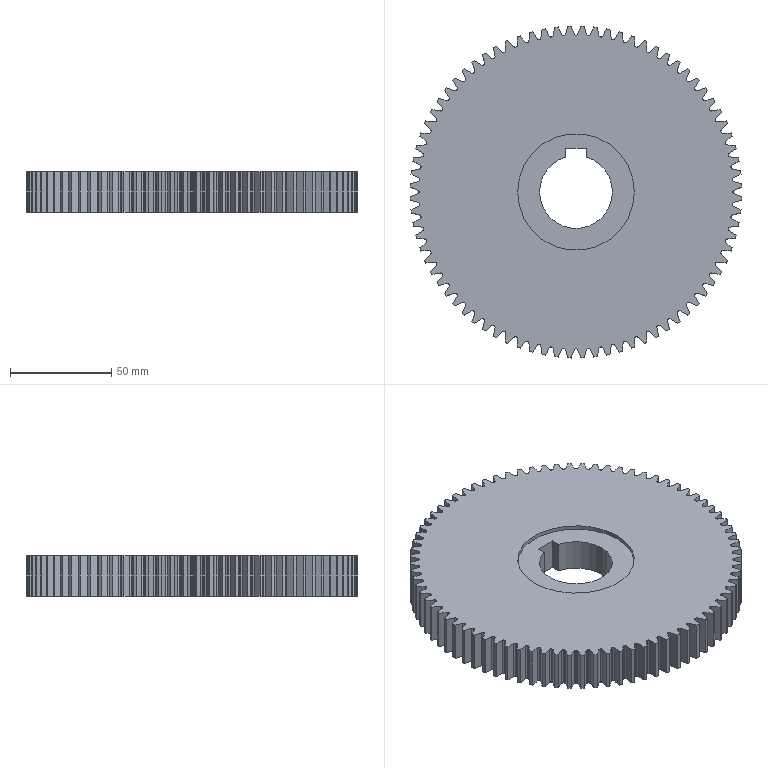Part | SolidWorks | features ICE 4, Extrusion 1 | 1 solid | 529 faces | box 163.929 x 163.929 x 20 mm | volume 373573 mm3 | cylinder 362 | spline 160 | plane 7 | commonest cylinder face diameters 1.52 x194 155 x81 164 x80 57.6 x4 36 x3